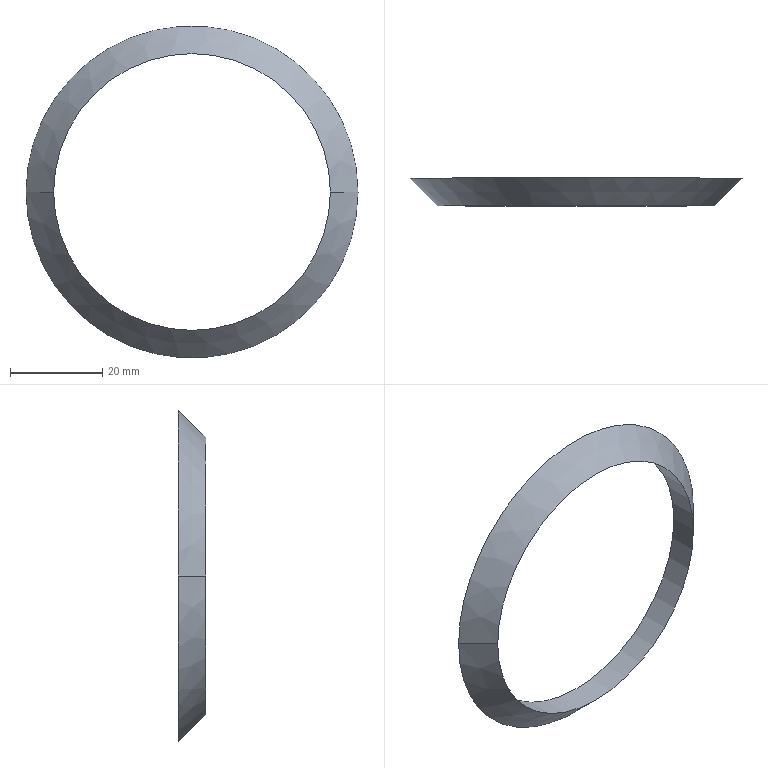Part | SolidWorks | 1 solid | 5 faces | box 72 x 6 x 72 mm | volume 3619 mm3 | cylinder 2 | cone 2 | plane 1 | commonest cylinder face diameters 60 x2
STEP:
#1=CARTESIAN_POINT('',(34.799,40.795,0.));
#2=VERTEX_POINT('',#1);
#3=CARTESIAN_POINT('',(-25.201,40.795,0.));
#4=VERTEX_POINT('',#3);
#5=CARTESIAN_POINT('',(4.799,40.795,0.));
#6=DIRECTION('',(0.,1.,0.));
#7=DIRECTION('',(1.,0.,0.));
#8=AXIS2_PLACEMENT_3D('',#5,#6,#7);
#9=CIRCLE('',#8,30.);
#10=EDGE_CURVE('',#2,#4,#9,.T.);
#11=ORIENTED_EDGE('',*,*,#10,.F.);
#12=CARTESIAN_POINT('',(4.799,40.795,0.));
#13=DIRECTION('',(0.,1.,0.));
#14=DIRECTION('',(-1.,0.,0.));
#15=AXIS2_PLACEMENT_3D('',#12,#13,#14);
#16=CIRCLE('',#15,30.);
#17=EDGE_CURVE('',#4,#2,#16,.T.);
#18=ORIENTED_EDGE('',*,*,#17,.F.);
#19=EDGE_LOOP('',(#11,#18));
#20=FACE_BOUND('',#19,.T.);
#21=CARTESIAN_POINT('',(40.799,40.795,0.));
#22=VERTEX_POINT('',#21);
#23=CARTESIAN_POINT('',(-31.201,40.795,0.));
#24=VERTEX_POINT('',#23);
#25=CARTESIAN_POINT('',(4.799,40.795,0.));
#26=DIRECTION('',(0.,-1.,0.));
#27=DIRECTION('',(1.,0.,0.));
#28=AXIS2_PLACEMENT_3D('',#25,#26,#27);
#29=CIRCLE('',#28,36.);
#30=EDGE_CURVE('',#22,#24,#29,.T.);
#31=ORIENTED_EDGE('',*,*,#30,.F.);
#32=CARTESIAN_POINT('',(4.799,40.795,0.));
#33=DIRECTION('',(0.,-1.,0.));
#34=DIRECTION('',(-1.,0.,0.));
#35=AXIS2_PLACEMENT_3D('',#32,#33,#34);
#36=CIRCLE('',#35,36.);
#37=EDGE_CURVE('',#24,#22,#36,.T.);
#38=ORIENTED_EDGE('',*,*,#37,.F.);
#39=EDGE_LOOP('',(#31,#38));
#40=FACE_OUTER_BOUND('',#39,.T.);
#41=CARTESIAN_POINT('',(4.799,40.795,0.));
#42=DIRECTION('',(0.,-1.,0.));
#43=DIRECTION('',(0.,0.,-1.));
#44=AXIS2_PLACEMENT_3D('',#41,#42,#43);
#45=PLANE('',#44);
#46=ADVANCED_FACE('',(#20,#40),#45,.F.);
#47=ORIENTED_EDGE('',*,*,#17,.T.);
#48=CARTESIAN_POINT('',(34.799,34.795,0.));
#49=VERTEX_POINT('',#48);
#50=CARTESIAN_POINT('',(34.799,40.795,0.));
#51=DIRECTION('',(0.,-1.,0.));
#52=VECTOR('',#51,1000.);
#53=LINE('',#50,#52);
#54=EDGE_CURVE('',#2,#49,#53,.T.);
#55=ORIENTED_EDGE('',*,*,#54,.T.);
#56=CARTESIAN_POINT('',(-25.201,34.795,0.));
#57=VERTEX_POINT('',#56);
#58=CARTESIAN_POINT('',(4.799,34.795,0.));
#59=DIRECTION('',(0.,-1.,0.));
#60=DIRECTION('',(1.,0.,0.));
#61=AXIS2_PLACEMENT_3D('',#58,#59,#60);
#62=CIRCLE('',#61,30.);
#63=EDGE_CURVE('',#49,#57,#62,.T.);
#64=ORIENTED_EDGE('',*,*,#63,.T.);
#65=CARTESIAN_POINT('',(-25.201,40.795,0.));
#66=DIRECTION('',(0.,-1.,0.));
#67=VECTOR('',#66,1000.);
#68=LINE('',#65,#67);
#69=EDGE_CURVE('',#4,#57,#68,.T.);
#70=ORIENTED_EDGE('',*,*,#69,.F.);
#71=EDGE_LOOP('',(#47,#55,#64,#70));
#72=FACE_OUTER_BOUND('',#71,.T.);
#73=CARTESIAN_POINT('',(4.799,-21.205,0.));
#74=DIRECTION('',(0.,1.,0.));
#75=DIRECTION('',(1.,0.,0.));
#76=AXIS2_PLACEMENT_3D('',#73,#74,#75);
#77=CYLINDRICAL_SURFACE('',#76,30.);
#78=ADVANCED_FACE('',(#72),#77,.F.);
#79=CARTESIAN_POINT('',(40.799,40.795,0.));
#80=DIRECTION('',(-0.7071,-0.7071,0.));
#81=VECTOR('',#80,1000.);
#82=LINE('',#79,#81);
#83=EDGE_CURVE('',#22,#49,#82,.T.);
#84=ORIENTED_EDGE('',*,*,#83,.F.);
#85=ORIENTED_EDGE('',*,*,#30,.T.);
#86=CARTESIAN_POINT('',(-31.201,40.795,0.));
#87=DIRECTION('',(0.7071,-0.7071,0.));
#88=VECTOR('',#87,1000.);
#89=LINE('',#86,#88);
#90=EDGE_CURVE('',#24,#57,#89,.T.);
#91=ORIENTED_EDGE('',*,*,#90,.T.);
#92=ORIENTED_EDGE('',*,*,#63,.F.);
#93=EDGE_LOOP('',(#84,#85,#91,#92));
#94=FACE_OUTER_BOUND('',#93,.T.);
#95=CARTESIAN_POINT('',(4.799,34.675,0.));
#96=DIRECTION('',(0.,1.,0.));
#97=DIRECTION('',(1.,0.,0.));
#98=AXIS2_PLACEMENT_3D('',#95,#96,#97);
#99=CONICAL_SURFACE('',#98,29.88,0.7854);
#100=ADVANCED_FACE('',(#94),#99,.T.);
#101=ORIENTED_EDGE('',*,*,#37,.T.);
#102=ORIENTED_EDGE('',*,*,#83,.T.);
#103=CARTESIAN_POINT('',(4.799,34.795,0.));
#104=DIRECTION('',(0.,-1.,0.));
#105=DIRECTION('',(-1.,0.,0.));
#106=AXIS2_PLACEMENT_3D('',#103,#104,#105);
#107=CIRCLE('',#106,30.);
#108=EDGE_CURVE('',#57,#49,#107,.T.);
#109=ORIENTED_EDGE('',*,*,#108,.F.);
#110=ORIENTED_EDGE('',*,*,#90,.F.);
#111=EDGE_LOOP('',(#101,#102,#109,#110));
#112=FACE_OUTER_BOUND('',#111,.T.);
#113=CARTESIAN_POINT('',(4.799,34.675,0.));
#114=DIRECTION('',(0.,1.,0.));
#115=DIRECTION('',(1.,0.,0.));
#116=AXIS2_PLACEMENT_3D('',#113,#114,#115);
#117=CONICAL_SURFACE('',#116,29.88,0.7854);
#118=ADVANCED_FACE('',(#112),#117,.T.);
#119=ORIENTED_EDGE('',*,*,#54,.F.);
#120=ORIENTED_EDGE('',*,*,#10,.T.);
#121=ORIENTED_EDGE('',*,*,#69,.T.);
#122=ORIENTED_EDGE('',*,*,#108,.T.);
#123=EDGE_LOOP('',(#119,#120,#121,#122));
#124=FACE_OUTER_BOUND('',#123,.T.);
#125=CARTESIAN_POINT('',(4.799,-21.205,0.));
#126=DIRECTION('',(0.,1.,0.));
#127=DIRECTION('',(1.,0.,0.));
#128=AXIS2_PLACEMENT_3D('',#125,#126,#127);
#129=CYLINDRICAL_SURFACE('',#128,30.);
#130=ADVANCED_FACE('',(#124),#129,.F.);
#131=CLOSED_SHELL('',(#46,#78,#100,#118,#130));
#132=MANIFOLD_SOLID_BREP('',#131);
#133=CARTESIAN_POINT('',(0.,0.,0.));
#134=DIRECTION('',(0.,0.,1.));
#135=DIRECTION('',(1.,0.,0.));
#136=AXIS2_PLACEMENT_3D('',#133,#134,#135);
#137=(LENGTH_UNIT()NAMED_UNIT(*)SI_UNIT(.MILLI.,.METRE.));
#138=UNCERTAINTY_MEASURE_WITH_UNIT(LENGTH_MEASURE(0.00001),#137,'','');
#139=(NAMED_UNIT(*)PLANE_ANGLE_UNIT()SI_UNIT($,.RADIAN.));
#140=(NAMED_UNIT(*)SI_UNIT($,.STERADIAN.)SOLID_ANGLE_UNIT());
#141=(GEOMETRIC_REPRESENTATION_CONTEXT(3)GLOBAL_UNCERTAINTY_ASSIGNED_CONTEXT((#138))GLOBAL_UNIT_ASSIGNED_CONTEXT((#137,#139,#140))REPRESENTATION_CONTEXT('',''));
#142=ADVANCED_BREP_SHAPE_REPRESENTATION('',(#132,#136),#141);